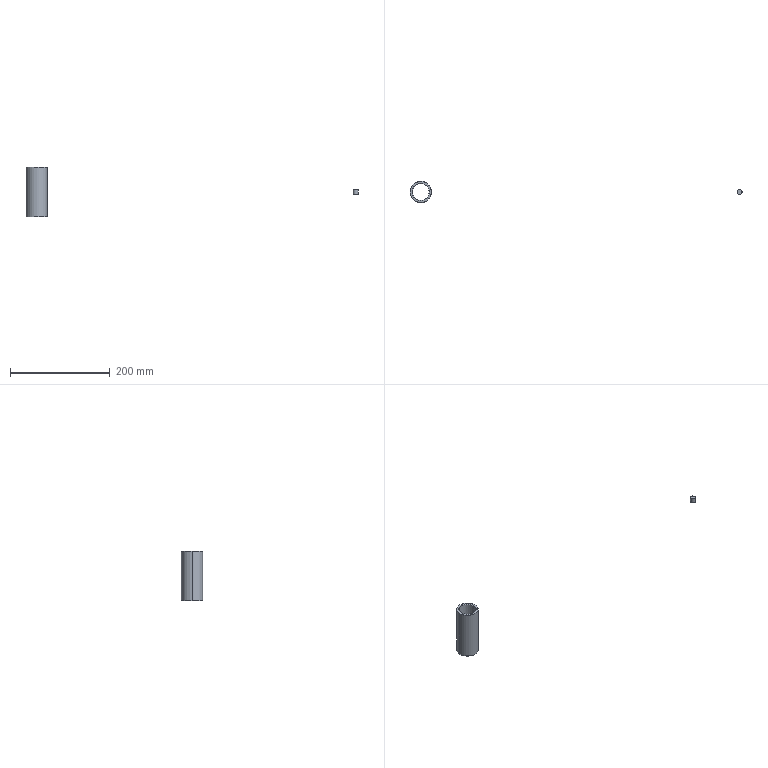Part | STEP file | PRT0001_68_8 | 2 solids | 18 faces | box 664.5 x 43 x 100 mm | volume 56748 mm3 | cone 8 | cylinder 6 | plane 4 | commonest cylinder face diameters 10 x2 33.7 x2 43 x2